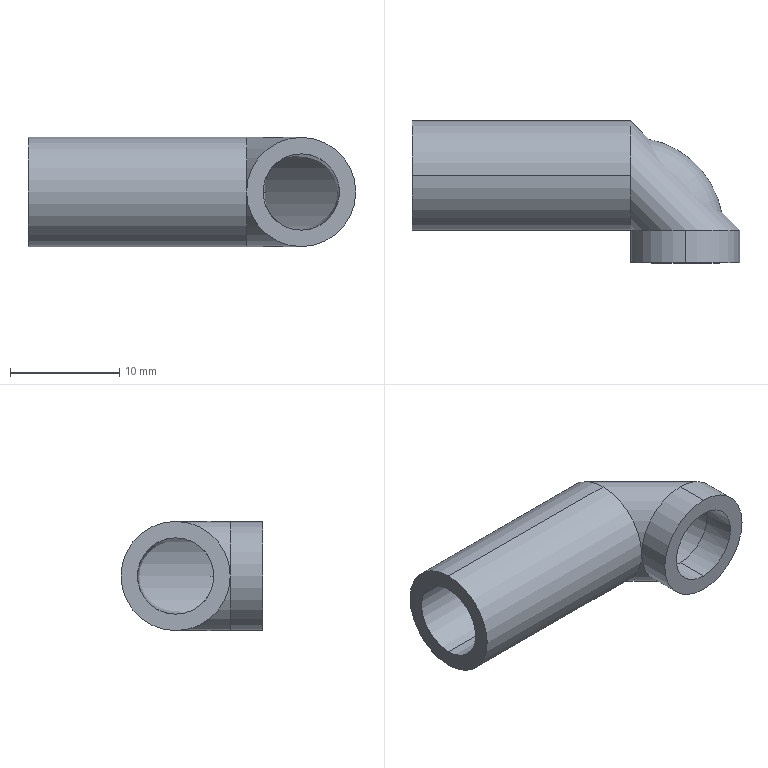Part | SolidWorks | features BaseBody 1 | 1 solid | 13 faces | box 30 x 13 x 10 mm | volume 1236 mm3 | cylinder 8 | torus 3 | plane 2 | commonest cylinder face diameters 7 x4 10 x4
STEP:
#1=CARTESIAN_POINT('',(20.,0.,3.5));
#2=VERTEX_POINT('',#1);
#3=CARTESIAN_POINT('',(20.,3.5,0.));
#4=VERTEX_POINT('',#3);
#5=CARTESIAN_POINT('',(20.,0.,0.));
#6=DIRECTION('',(-1.,0.,0.));
#7=DIRECTION('',(0.,0.,-1.));
#8=AXIS2_PLACEMENT_3D('',#5,#6,#7);
#9=CIRCLE('',#8,3.5);
#10=EDGE_CURVE('',#2,#4,#9,.T.);
#11=ORIENTED_EDGE('',*,*,#10,.T.);
#12=CARTESIAN_POINT('',(28.5,-5.,0.));
#13=VERTEX_POINT('',#12);
#14=CARTESIAN_POINT('',(20.,-5.,0.));
#15=DIRECTION('',(0.,0.,-1.));
#16=DIRECTION('',(-1.,0.,0.));
#17=AXIS2_PLACEMENT_3D('',#14,#15,#16);
#18=CIRCLE('',#17,8.5);
#19=EDGE_CURVE('',#4,#13,#18,.T.);
#20=ORIENTED_EDGE('',*,*,#19,.T.);
#21=CARTESIAN_POINT('',(25.,-5.,3.5));
#22=VERTEX_POINT('',#21);
#23=CARTESIAN_POINT('',(25.,-5.,0.));
#24=DIRECTION('',(0.00001962,1.,0.));
#25=DIRECTION('',(0.,0.,-1.));
#26=AXIS2_PLACEMENT_3D('',#23,#24,#25);
#27=CIRCLE('',#26,3.5);
#28=EDGE_CURVE('',#22,#13,#27,.T.);
#29=ORIENTED_EDGE('',*,*,#28,.F.);
#30=CARTESIAN_POINT('',(21.5,-5.,0.));
#31=VERTEX_POINT('',#30);
#32=CARTESIAN_POINT('',(25.,-5.,0.));
#33=DIRECTION('',(0.00001962,1.,0.));
#34=DIRECTION('',(0.,0.,-1.));
#35=AXIS2_PLACEMENT_3D('',#32,#33,#34);
#36=CIRCLE('',#35,3.5);
#37=EDGE_CURVE('',#31,#22,#36,.T.);
#38=ORIENTED_EDGE('',*,*,#37,.F.);
#39=CARTESIAN_POINT('',(20.,-3.5,0.));
#40=VERTEX_POINT('',#39);
#41=CARTESIAN_POINT('',(20.,-5.,0.));
#42=DIRECTION('',(0.,0.,-1.));
#43=DIRECTION('',(-1.,0.,0.));
#44=AXIS2_PLACEMENT_3D('',#41,#42,#43);
#45=CIRCLE('',#44,1.5);
#46=EDGE_CURVE('',#40,#31,#45,.T.);
#47=ORIENTED_EDGE('',*,*,#46,.F.);
#48=CARTESIAN_POINT('',(20.,0.,0.));
#49=DIRECTION('',(-1.,0.,0.));
#50=DIRECTION('',(0.,0.,-1.));
#51=AXIS2_PLACEMENT_3D('',#48,#49,#50);
#52=CIRCLE('',#51,3.5);
#53=EDGE_CURVE('',#40,#2,#52,.T.);
#54=ORIENTED_EDGE('',*,*,#53,.T.);
#55=EDGE_LOOP('',(#11,#20,#29,#38,#47,#54));
#56=FACE_OUTER_BOUND('',#55,.T.);
#57=CARTESIAN_POINT('',(20.,-5.,0.));
#58=DIRECTION('',(0.,0.,-1.));
#59=DIRECTION('',(-1.,0.,0.));
#60=AXIS2_PLACEMENT_3D('',#57,#58,#59);
#61=TOROIDAL_SURFACE('',#60,5.,3.5);
#62=ADVANCED_FACE('',(#56),#61,.F.);
#63=CARTESIAN_POINT('',(0.,0.,-3.5));
#64=VERTEX_POINT('',#63);
#65=CARTESIAN_POINT('',(0.,0.,3.5));
#66=VERTEX_POINT('',#65);
#67=CARTESIAN_POINT('',(0.,0.,0.));
#68=DIRECTION('',(-1.,0.,0.));
#69=DIRECTION('',(0.,0.,-1.));
#70=AXIS2_PLACEMENT_3D('',#67,#68,#69);
#71=CIRCLE('',#70,3.5);
#72=EDGE_CURVE('',#64,#66,#71,.T.);
#73=ORIENTED_EDGE('',*,*,#72,.T.);
#74=CARTESIAN_POINT('',(0.,0.,3.5));
#75=DIRECTION('',(1.,0.,0.));
#76=VECTOR('',#75,1000.);
#77=LINE('',#74,#76);
#78=EDGE_CURVE('',#66,#2,#77,.T.);
#79=ORIENTED_EDGE('',*,*,#78,.T.);
#80=ORIENTED_EDGE('',*,*,#53,.F.);
#81=CARTESIAN_POINT('',(20.,0.,-3.5));
#82=VERTEX_POINT('',#81);
#83=CARTESIAN_POINT('',(20.,0.,0.));
#84=DIRECTION('',(-1.,0.,0.));
#85=DIRECTION('',(0.,0.,-1.));
#86=AXIS2_PLACEMENT_3D('',#83,#84,#85);
#87=CIRCLE('',#86,3.5);
#88=EDGE_CURVE('',#82,#40,#87,.T.);
#89=ORIENTED_EDGE('',*,*,#88,.F.);
#90=CARTESIAN_POINT('',(0.,0.,-3.5));
#91=DIRECTION('',(1.,0.,0.));
#92=VECTOR('',#91,1000.);
#93=LINE('',#90,#92);
#94=EDGE_CURVE('',#64,#82,#93,.T.);
#95=ORIENTED_EDGE('',*,*,#94,.F.);
#96=EDGE_LOOP('',(#73,#79,#80,#89,#95));
#97=FACE_OUTER_BOUND('',#96,.T.);
#98=CARTESIAN_POINT('',(0.,0.,0.));
#99=DIRECTION('',(1.,0.,0.));
#100=DIRECTION('',(0.,0.,-1.));
#101=AXIS2_PLACEMENT_3D('',#98,#99,#100);
#102=CYLINDRICAL_SURFACE('',#101,3.5);
#103=ADVANCED_FACE('',(#97),#102,.F.);
#104=CARTESIAN_POINT('',(25.,-5.,-3.5));
#105=VERTEX_POINT('',#104);
#106=CARTESIAN_POINT('',(25.,-5.,0.));
#107=DIRECTION('',(0.00001962,1.,0.));
#108=DIRECTION('',(0.,0.,-1.));
#109=AXIS2_PLACEMENT_3D('',#106,#107,#108);
#110=CIRCLE('',#109,3.5);
#111=EDGE_CURVE('',#105,#31,#110,.T.);
#112=ORIENTED_EDGE('',*,*,#111,.T.);
#113=ORIENTED_EDGE('',*,*,#37,.T.);
#114=CARTESIAN_POINT('',(25.,-8.,3.5));
#115=VERTEX_POINT('',#114);
#116=CARTESIAN_POINT('',(25.,-5.,3.5));
#117=DIRECTION('',(0.,-1.,0.));
#118=VECTOR('',#117,1000.);
#119=LINE('',#116,#118);
#120=EDGE_CURVE('',#22,#115,#119,.T.);
#121=ORIENTED_EDGE('',*,*,#120,.T.);
#122=CARTESIAN_POINT('',(25.,-8.,-3.5));
#123=VERTEX_POINT('',#122);
#124=CARTESIAN_POINT('',(25.,-8.,0.));
#125=DIRECTION('',(0.,1.,0.));
#126=DIRECTION('',(0.,0.,-1.));
#127=AXIS2_PLACEMENT_3D('',#124,#125,#126);
#128=CIRCLE('',#127,3.5);
#129=EDGE_CURVE('',#123,#115,#128,.T.);
#130=ORIENTED_EDGE('',*,*,#129,.F.);
#131=CARTESIAN_POINT('',(25.,-5.,-3.5));
#132=DIRECTION('',(0.,-1.,0.));
#133=VECTOR('',#132,1000.);
#134=LINE('',#131,#133);
#135=EDGE_CURVE('',#105,#123,#134,.T.);
#136=ORIENTED_EDGE('',*,*,#135,.F.);
#137=EDGE_LOOP('',(#112,#113,#121,#130,#136));
#138=FACE_OUTER_BOUND('',#137,.T.);
#139=CARTESIAN_POINT('',(25.,-5.,0.));
#140=DIRECTION('',(0.,-1.,0.));
#141=DIRECTION('',(0.,0.,-1.));
#142=AXIS2_PLACEMENT_3D('',#139,#140,#141);
#143=CYLINDRICAL_SURFACE('',#142,3.5);
#144=ADVANCED_FACE('',(#138),#143,.F.);
#145=CARTESIAN_POINT('',(0.,0.,-5.));
#146=VERTEX_POINT('',#145);
#147=CARTESIAN_POINT('',(0.,0.,5.));
#148=VERTEX_POINT('',#147);
#149=CARTESIAN_POINT('',(0.,0.,0.));
#150=DIRECTION('',(1.,0.,0.));
#151=DIRECTION('',(0.,0.,-1.));
#152=AXIS2_PLACEMENT_3D('',#149,#150,#151);
#153=CIRCLE('',#152,5.);
#154=EDGE_CURVE('',#146,#148,#153,.T.);
#155=ORIENTED_EDGE('',*,*,#154,.T.);
#156=CARTESIAN_POINT('',(20.,0.,5.));
#157=VERTEX_POINT('',#156);
#158=CARTESIAN_POINT('',(0.,0.,5.));
#159=DIRECTION('',(1.,0.,0.));
#160=VECTOR('',#159,1000.);
#161=LINE('',#158,#160);
#162=EDGE_CURVE('',#148,#157,#161,.T.);
#163=ORIENTED_EDGE('',*,*,#162,.T.);
#164=CARTESIAN_POINT('',(20.,0.,-5.));
#165=VERTEX_POINT('',#164);
#166=CARTESIAN_POINT('',(20.,0.,0.));
#167=DIRECTION('',(1.,0.,0.));
#168=DIRECTION('',(0.,0.,-1.));
#169=AXIS2_PLACEMENT_3D('',#166,#167,#168);
#170=CIRCLE('',#169,5.);
#171=EDGE_CURVE('',#165,#157,#170,.T.);
#172=ORIENTED_EDGE('',*,*,#171,.F.);
#173=CARTESIAN_POINT('',(0.,0.,-5.));
#174=DIRECTION('',(1.,0.,0.));
#175=VECTOR('',#174,1000.);
#176=LINE('',#173,#175);
#177=EDGE_CURVE('',#146,#165,#176,.T.);
#178=ORIENTED_EDGE('',*,*,#177,.F.);
#179=EDGE_LOOP('',(#155,#163,#172,#178));
#180=FACE_OUTER_BOUND('',#179,.T.);
#181=CARTESIAN_POINT('',(0.,0.,0.));
#182=DIRECTION('',(1.,0.,0.));
#183=DIRECTION('',(0.,0.,-1.));
#184=AXIS2_PLACEMENT_3D('',#181,#182,#183);
#185=CYLINDRICAL_SURFACE('',#184,5.);
#186=ADVANCED_FACE('',(#180),#185,.T.);
#187=CARTESIAN_POINT('',(25.,-5.,-5.));
#188=VERTEX_POINT('',#187);
#189=CARTESIAN_POINT('',(25.,-5.,5.));
#190=VERTEX_POINT('',#189);
#191=CARTESIAN_POINT('',(25.,-5.,0.));
#192=DIRECTION('',(-0.00001962,-1.,0.));
#193=DIRECTION('',(0.,0.,-1.));
#194=AXIS2_PLACEMENT_3D('',#191,#192,#193);
#195=CIRCLE('',#194,5.);
#196=EDGE_CURVE('',#188,#190,#195,.T.);
#197=ORIENTED_EDGE('',*,*,#196,.T.);
#198=CARTESIAN_POINT('',(25.,-8.,5.));
#199=VERTEX_POINT('',#198);
#200=CARTESIAN_POINT('',(25.,-5.,5.));
#201=DIRECTION('',(0.,-1.,0.));
#202=VECTOR('',#201,1000.);
#203=LINE('',#200,#202);
#204=EDGE_CURVE('',#190,#199,#203,.T.);
#205=ORIENTED_EDGE('',*,*,#204,.T.);
#206=CARTESIAN_POINT('',(25.,-8.,-5.));
#207=VERTEX_POINT('',#206);
#208=CARTESIAN_POINT('',(25.,-8.,0.));
#209=DIRECTION('',(0.,-1.,0.));
#210=DIRECTION('',(0.,0.,-1.));
#211=AXIS2_PLACEMENT_3D('',#208,#209,#210);
#212=CIRCLE('',#211,5.);
#213=EDGE_CURVE('',#207,#199,#212,.T.);
#214=ORIENTED_EDGE('',*,*,#213,.F.);
#215=CARTESIAN_POINT('',(25.,-5.,-5.));
#216=DIRECTION('',(0.,-1.,0.));
#217=VECTOR('',#216,1000.);
#218=LINE('',#215,#217);
#219=EDGE_CURVE('',#188,#207,#218,.T.);
#220=ORIENTED_EDGE('',*,*,#219,.F.);
#221=EDGE_LOOP('',(#197,#205,#214,#220));
#222=FACE_OUTER_BOUND('',#221,.T.);
#223=CARTESIAN_POINT('',(25.,-5.,0.));
#224=DIRECTION('',(0.,-1.,0.));
#225=DIRECTION('',(0.,0.,-1.));
#226=AXIS2_PLACEMENT_3D('',#223,#224,#225);
#227=CYLINDRICAL_SURFACE('',#226,5.);
#228=ADVANCED_FACE('',(#222),#227,.T.);
#229=ORIENTED_EDGE('',*,*,#204,.F.);
#230=CARTESIAN_POINT('',(20.,-5.,0.));
#231=VERTEX_POINT('',#230);
#232=CARTESIAN_POINT('',(25.,-5.,0.));
#233=DIRECTION('',(-0.00001962,-1.,0.));
#234=DIRECTION('',(0.,0.,-1.));
#235=AXIS2_PLACEMENT_3D('',#232,#233,#234);
#236=CIRCLE('',#235,5.);
#237=EDGE_CURVE('',#190,#231,#236,.T.);
#238=ORIENTED_EDGE('',*,*,#237,.T.);
#239=CARTESIAN_POINT('',(25.,-5.,0.));
#240=DIRECTION('',(-0.00001962,-1.,0.));
#241=DIRECTION('',(0.,0.,-1.));
#242=AXIS2_PLACEMENT_3D('',#239,#240,#241);
#243=CIRCLE('',#242,5.);
#244=EDGE_CURVE('',#231,#188,#243,.T.);
#245=ORIENTED_EDGE('',*,*,#244,.T.);
#246=ORIENTED_EDGE('',*,*,#219,.T.);
#247=CARTESIAN_POINT('',(25.,-8.,0.));
#248=DIRECTION('',(0.,-1.,0.));
#249=DIRECTION('',(0.,0.,-1.));
#250=AXIS2_PLACEMENT_3D('',#247,#248,#249);
#251=CIRCLE('',#250,5.);
#252=EDGE_CURVE('',#199,#207,#251,.T.);
#253=ORIENTED_EDGE('',*,*,#252,.F.);
#254=EDGE_LOOP('',(#229,#238,#245,#246,#253));
#255=FACE_OUTER_BOUND('',#254,.T.);
#256=CARTESIAN_POINT('',(25.,-5.,0.));
#257=DIRECTION('',(0.,-1.,0.));
#258=DIRECTION('',(0.,0.,-1.));
#259=AXIS2_PLACEMENT_3D('',#256,#257,#258);
#260=CYLINDRICAL_SURFACE('',#259,5.);
#261=ADVANCED_FACE('',(#255),#260,.T.);
#262=ORIENTED_EDGE('',*,*,#162,.F.);
#263=CARTESIAN_POINT('',(0.,0.,0.));
#264=DIRECTION('',(1.,0.,0.));
#265=DIRECTION('',(0.,0.,-1.));
#266=AXIS2_PLACEMENT_3D('',#263,#264,#265);
#267=CIRCLE('',#266,5.);
#268=EDGE_CURVE('',#148,#146,#267,.T.);
#269=ORIENTED_EDGE('',*,*,#268,.T.);
#270=ORIENTED_EDGE('',*,*,#177,.T.);
#271=CARTESIAN_POINT('',(20.,0.,0.));
#272=DIRECTION('',(1.,0.,0.));
#273=DIRECTION('',(0.,0.,-1.));
#274=AXIS2_PLACEMENT_3D('',#271,#272,#273);
#275=CIRCLE('',#274,5.);
#276=EDGE_CURVE('',#231,#165,#275,.T.);
#277=ORIENTED_EDGE('',*,*,#276,.F.);
#278=CARTESIAN_POINT('',(20.,0.,0.));
#279=DIRECTION('',(1.,0.,0.));
#280=DIRECTION('',(0.,0.,-1.));
#281=AXIS2_PLACEMENT_3D('',#278,#279,#280);
#282=CIRCLE('',#281,5.);
#283=EDGE_CURVE('',#157,#231,#282,.T.);
#284=ORIENTED_EDGE('',*,*,#283,.F.);
#285=EDGE_LOOP('',(#262,#269,#270,#277,#284));
#286=FACE_OUTER_BOUND('',#285,.T.);
#287=CARTESIAN_POINT('',(0.,0.,0.));
#288=DIRECTION('',(1.,0.,0.));
#289=DIRECTION('',(0.,0.,-1.));
#290=AXIS2_PLACEMENT_3D('',#287,#288,#289);
#291=CYLINDRICAL_SURFACE('',#290,5.);
#292=ADVANCED_FACE('',(#286),#291,.T.);
#293=ORIENTED_EDGE('',*,*,#244,.F.);
#294=ORIENTED_EDGE('',*,*,#276,.T.);
#295=ORIENTED_EDGE('',*,*,#171,.T.);
#296=ORIENTED_EDGE('',*,*,#283,.T.);
#297=ORIENTED_EDGE('',*,*,#237,.F.);
#298=ORIENTED_EDGE('',*,*,#196,.F.);
#299=EDGE_LOOP('',(#293,#294,#295,#296,#297,#298));
#300=FACE_OUTER_BOUND('',#299,.T.);
#301=CARTESIAN_POINT('',(20.,-5.,0.));
#302=DIRECTION('',(0.,0.,-1.));
#303=DIRECTION('',(-1.,0.,0.));
#304=AXIS2_PLACEMENT_3D('',#301,#302,#303);
#305=TOROIDAL_SURFACE('',#304,5.,5.);
#306=ADVANCED_FACE('',(#300),#305,.T.);
#307=ORIENTED_EDGE('',*,*,#129,.T.);
#308=CARTESIAN_POINT('',(25.,-8.,0.));
#309=DIRECTION('',(0.,1.,0.));
#310=DIRECTION('',(0.,0.,-1.));
#311=AXIS2_PLACEMENT_3D('',#308,#309,#310);
#312=CIRCLE('',#311,3.5);
#313=EDGE_CURVE('',#115,#123,#312,.T.);
#314=ORIENTED_EDGE('',*,*,#313,.T.);
#315=EDGE_LOOP('',(#307,#314));
#316=FACE_BOUND('',#315,.T.);
#317=ORIENTED_EDGE('',*,*,#213,.T.);
#318=ORIENTED_EDGE('',*,*,#252,.T.);
#319=EDGE_LOOP('',(#317,#318));
#320=FACE_OUTER_BOUND('',#319,.T.);
#321=CARTESIAN_POINT('',(25.,-8.,0.));
#322=DIRECTION('',(0.,-1.,0.));
#323=DIRECTION('',(0.,0.,-1.));
#324=AXIS2_PLACEMENT_3D('',#321,#322,#323);
#325=PLANE('',#324);
#326=ADVANCED_FACE('',(#316,#320),#325,.T.);
#327=ORIENTED_EDGE('',*,*,#72,.F.);
#328=CARTESIAN_POINT('',(0.,0.,0.));
#329=DIRECTION('',(-1.,0.,0.));
#330=DIRECTION('',(0.,0.,-1.));
#331=AXIS2_PLACEMENT_3D('',#328,#329,#330);
#332=CIRCLE('',#331,3.5);
#333=EDGE_CURVE('',#66,#64,#332,.T.);
#334=ORIENTED_EDGE('',*,*,#333,.F.);
#335=EDGE_LOOP('',(#327,#334));
#336=FACE_BOUND('',#335,.T.);
#337=ORIENTED_EDGE('',*,*,#154,.F.);
#338=ORIENTED_EDGE('',*,*,#268,.F.);
#339=EDGE_LOOP('',(#337,#338));
#340=FACE_OUTER_BOUND('',#339,.T.);
#341=CARTESIAN_POINT('',(0.,0.,0.));
#342=DIRECTION('',(1.,0.,0.));
#343=DIRECTION('',(0.,0.,-1.));
#344=AXIS2_PLACEMENT_3D('',#341,#342,#343);
#345=PLANE('',#344);
#346=ADVANCED_FACE('',(#336,#340),#345,.F.);
#347=ORIENTED_EDGE('',*,*,#120,.F.);
#348=ORIENTED_EDGE('',*,*,#28,.T.);
#349=CARTESIAN_POINT('',(25.,-5.,0.));
#350=DIRECTION('',(0.00001962,1.,0.));
#351=DIRECTION('',(0.,0.,-1.));
#352=AXIS2_PLACEMENT_3D('',#349,#350,#351);
#353=CIRCLE('',#352,3.5);
#354=EDGE_CURVE('',#13,#105,#353,.T.);
#355=ORIENTED_EDGE('',*,*,#354,.T.);
#356=ORIENTED_EDGE('',*,*,#135,.T.);
#357=ORIENTED_EDGE('',*,*,#313,.F.);
#358=EDGE_LOOP('',(#347,#348,#355,#356,#357));
#359=FACE_OUTER_BOUND('',#358,.T.);
#360=CARTESIAN_POINT('',(25.,-5.,0.));
#361=DIRECTION('',(0.,-1.,0.));
#362=DIRECTION('',(0.,0.,-1.));
#363=AXIS2_PLACEMENT_3D('',#360,#361,#362);
#364=CYLINDRICAL_SURFACE('',#363,3.5);
#365=ADVANCED_FACE('',(#359),#364,.F.);
#366=ORIENTED_EDGE('',*,*,#78,.F.);
#367=ORIENTED_EDGE('',*,*,#333,.T.);
#368=ORIENTED_EDGE('',*,*,#94,.T.);
#369=CARTESIAN_POINT('',(20.,0.,0.));
#370=DIRECTION('',(-1.,0.,0.));
#371=DIRECTION('',(0.,0.,-1.));
#372=AXIS2_PLACEMENT_3D('',#369,#370,#371);
#373=CIRCLE('',#372,3.5);
#374=EDGE_CURVE('',#4,#82,#373,.T.);
#375=ORIENTED_EDGE('',*,*,#374,.F.);
#376=ORIENTED_EDGE('',*,*,#10,.F.);
#377=EDGE_LOOP('',(#366,#367,#368,#375,#376));
#378=FACE_OUTER_BOUND('',#377,.T.);
#379=CARTESIAN_POINT('',(0.,0.,0.));
#380=DIRECTION('',(1.,0.,0.));
#381=DIRECTION('',(0.,0.,-1.));
#382=AXIS2_PLACEMENT_3D('',#379,#380,#381);
#383=CYLINDRICAL_SURFACE('',#382,3.5);
#384=ADVANCED_FACE('',(#378),#383,.F.);
#385=ORIENTED_EDGE('',*,*,#19,.F.);
#386=ORIENTED_EDGE('',*,*,#374,.T.);
#387=ORIENTED_EDGE('',*,*,#88,.T.);
#388=ORIENTED_EDGE('',*,*,#46,.T.);
#389=ORIENTED_EDGE('',*,*,#111,.F.);
#390=ORIENTED_EDGE('',*,*,#354,.F.);
#391=EDGE_LOOP('',(#385,#386,#387,#388,#389,#390));
#392=FACE_OUTER_BOUND('',#391,.T.);
#393=CARTESIAN_POINT('',(20.,-5.,0.));
#394=DIRECTION('',(0.,0.,-1.));
#395=DIRECTION('',(-1.,0.,0.));
#396=AXIS2_PLACEMENT_3D('',#393,#394,#395);
#397=TOROIDAL_SURFACE('',#396,5.,3.5);
#398=ADVANCED_FACE('',(#392),#397,.F.);
#399=CLOSED_SHELL('',(#62,#103,#144,#186,#228,#261,#292,#306,#326,#346,#365,#384,#398));
#400=MANIFOLD_SOLID_BREP('',#399);
#401=CARTESIAN_POINT('',(0.,0.,0.));
#402=DIRECTION('',(0.,0.,1.));
#403=DIRECTION('',(1.,0.,0.));
#404=AXIS2_PLACEMENT_3D('',#401,#402,#403);
#405=(LENGTH_UNIT()NAMED_UNIT(*)SI_UNIT(.MILLI.,.METRE.));
#406=UNCERTAINTY_MEASURE_WITH_UNIT(LENGTH_MEASURE(0.00001),#405,'','');
#407=(NAMED_UNIT(*)PLANE_ANGLE_UNIT()SI_UNIT($,.RADIAN.));
#408=(NAMED_UNIT(*)SI_UNIT($,.STERADIAN.)SOLID_ANGLE_UNIT());
#409=(GEOMETRIC_REPRESENTATION_CONTEXT(3)GLOBAL_UNCERTAINTY_ASSIGNED_CONTEXT((#406))GLOBAL_UNIT_ASSIGNED_CONTEXT((#405,#407,#408))REPRESENTATION_CONTEXT('',''));
#410=ADVANCED_BREP_SHAPE_REPRESENTATION('',(#400,#404),#409);